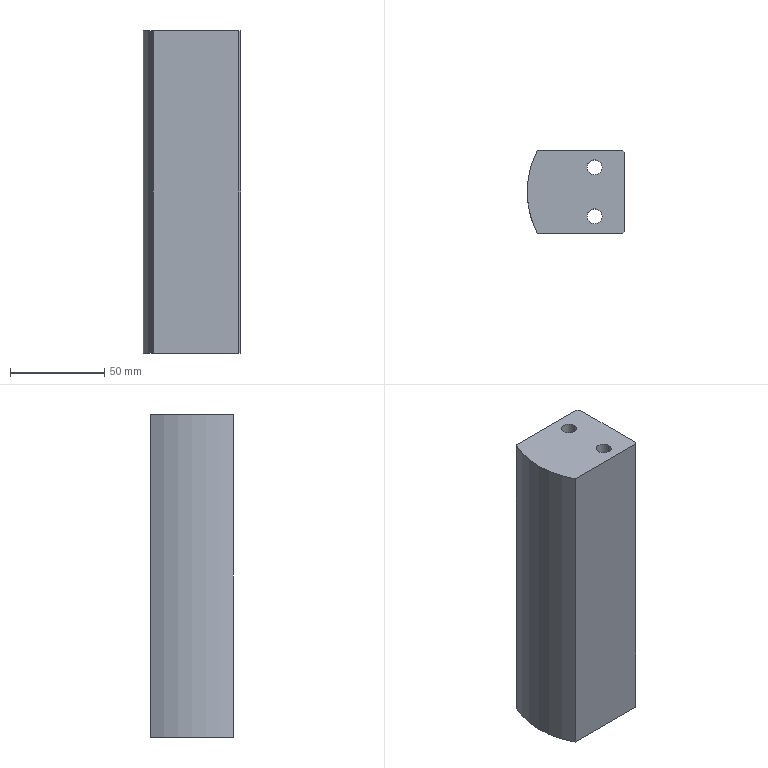Part | STEP file | 1 solid | 172 faces | box 51.8 x 44 x 171 mm | volume 352812 mm3 | cylinder 79 | cone 57 | plane 36 | commonest cylinder face diameters 4 x32 9 x32 3.2 x4 7 x4 8 x4 6.4 x2